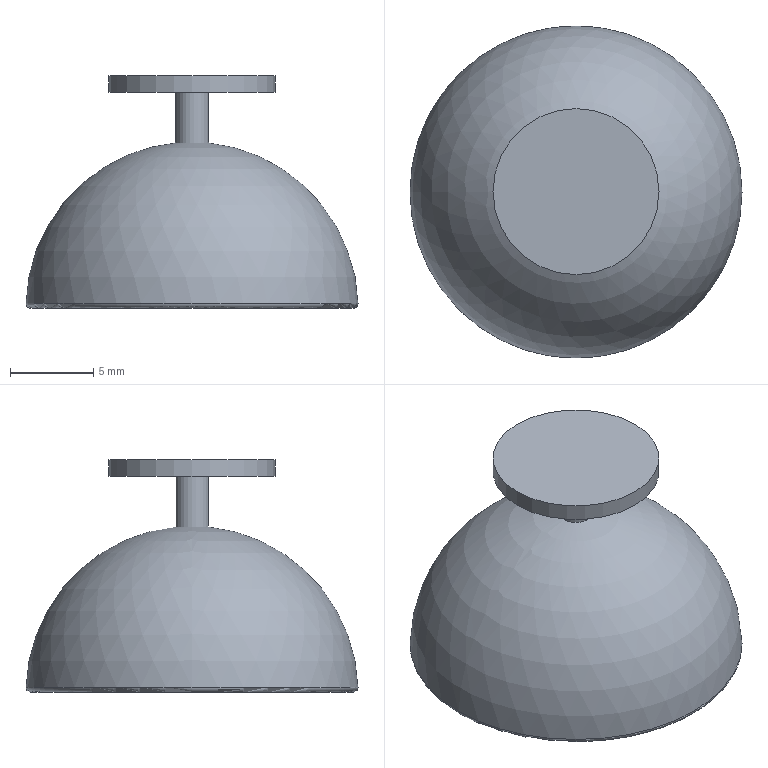Part | NX | features DATUM_CSYS 3, SKETCH 2, BLEND 1, REPLACE_FACE 1, SHELL 1, SPHERE 1, SWP104 1, TRIM BODY 1, UNITE 1 | 1 solid | 9 faces | box 19.991 x 19.991 x 14 mm | volume 1108 mm3 | plane 3 | sphere 2 | cylinder 2 | torus 2 | commonest cylinder face diameters 2 x1 10 x1
STEP:
#1=CARTESIAN_POINT('',(-9.995,0.,0.3093));
#2=VERTEX_POINT('',#1);
#3=CARTESIAN_POINT('',(0.,0.,0.3093));
#4=DIRECTION('',(0.,0.,-1.));
#5=DIRECTION('',(-1.,0.,0.));
#6=AXIS2_PLACEMENT_3D('',#3,#4,#5);
#7=CIRCLE('',#6,9.995);
#8=EDGE_CURVE('',#2,#2,#7,.F.);
#9=ORIENTED_EDGE('',*,*,#8,.T.);
#10=EDGE_LOOP('',(#9));
#11=FACE_BOUND('',#10,.T.);
#12=CARTESIAN_POINT('',(-1.,0.,9.95));
#13=VERTEX_POINT('',#12);
#14=CARTESIAN_POINT('',(0.,0.,9.95));
#15=DIRECTION('',(0.,0.,-1.));
#16=DIRECTION('',(-1.,0.,0.));
#17=AXIS2_PLACEMENT_3D('',#14,#15,#16);
#18=CIRCLE('',#17,1.);
#19=EDGE_CURVE('',#13,#13,#18,.T.);
#20=ORIENTED_EDGE('',*,*,#19,.T.);
#21=EDGE_LOOP('',(#20));
#22=FACE_BOUND('',#21,.T.);
#23=CARTESIAN_POINT('',(0.,0.,0.));
#24=DIRECTION('',(0.,0.,1.));
#25=DIRECTION('',(1.,0.,0.));
#26=AXIS2_PLACEMENT_3D('',#23,#24,#25);
#27=SPHERICAL_SURFACE('',#26,10.);
#28=ADVANCED_FACE('',(#11,#22),#27,.T.);
#29=CARTESIAN_POINT('',(-7.995,0.,0.2892));
#30=VERTEX_POINT('',#29);
#31=CARTESIAN_POINT('',(0.,0.,0.2892));
#32=DIRECTION('',(0.,0.,-1.));
#33=DIRECTION('',(-1.,0.,0.));
#34=AXIS2_PLACEMENT_3D('',#31,#32,#33);
#35=CIRCLE('',#34,7.995);
#36=EDGE_CURVE('',#30,#30,#35,.T.);
#37=ORIENTED_EDGE('',*,*,#36,.T.);
#38=EDGE_LOOP('',(#37));
#39=FACE_BOUND('',#38,.T.);
#40=CARTESIAN_POINT('',(0.,0.,0.));
#41=DIRECTION('',(0.,0.,1.));
#42=DIRECTION('',(1.,0.,0.));
#43=AXIS2_PLACEMENT_3D('',#40,#41,#42);
#44=SPHERICAL_SURFACE('',#43,8.);
#45=ADVANCED_FACE('',(#39),#44,.F.);
#46=CARTESIAN_POINT('',(8.295,0.,0.));
#47=VERTEX_POINT('',#46);
#48=CARTESIAN_POINT('',(0.,0.,0.));
#49=DIRECTION('',(0.,0.,1.));
#50=DIRECTION('',(1.,0.,0.));
#51=AXIS2_PLACEMENT_3D('',#48,#49,#50);
#52=CIRCLE('',#51,8.295);
#53=EDGE_CURVE('',#47,#47,#52,.T.);
#54=ORIENTED_EDGE('',*,*,#53,.T.);
#55=EDGE_LOOP('',(#54));
#56=FACE_BOUND('',#55,.T.);
#57=CARTESIAN_POINT('',(9.695,0.,0.));
#58=VERTEX_POINT('',#57);
#59=CARTESIAN_POINT('',(0.,0.,0.));
#60=DIRECTION('',(0.,0.,1.));
#61=DIRECTION('',(1.,0.,0.));
#62=AXIS2_PLACEMENT_3D('',#59,#60,#61);
#63=CIRCLE('',#62,9.695);
#64=EDGE_CURVE('',#58,#58,#63,.F.);
#65=ORIENTED_EDGE('',*,*,#64,.T.);
#66=EDGE_LOOP('',(#65));
#67=FACE_BOUND('',#66,.T.);
#68=CARTESIAN_POINT('',(0.,0.,0.));
#69=DIRECTION('',(0.,0.,1.));
#70=DIRECTION('',(1.,0.,0.));
#71=AXIS2_PLACEMENT_3D('',#68,#69,#70);
#72=PLANE('',#71);
#73=ADVANCED_FACE('',(#56,#67),#72,.F.);
#74=CARTESIAN_POINT('',(-5.,0.,14.));
#75=VERTEX_POINT('',#74);
#76=CARTESIAN_POINT('',(0.,0.,14.));
#77=DIRECTION('',(0.,0.,-1.));
#78=DIRECTION('',(-1.,0.,0.));
#79=AXIS2_PLACEMENT_3D('',#76,#77,#78);
#80=CIRCLE('',#79,5.);
#81=EDGE_CURVE('',#75,#75,#80,.T.);
#82=ORIENTED_EDGE('',*,*,#81,.F.);
#83=EDGE_LOOP('',(#82));
#84=FACE_BOUND('',#83,.T.);
#85=CARTESIAN_POINT('',(0.,0.,14.));
#86=DIRECTION('',(0.,0.,-1.));
#87=DIRECTION('',(-1.,0.,0.));
#88=AXIS2_PLACEMENT_3D('',#85,#86,#87);
#89=PLANE('',#88);
#90=ADVANCED_FACE('',(#84),#89,.F.);
#91=CARTESIAN_POINT('',(-5.,0.,13.));
#92=VERTEX_POINT('',#91);
#93=CARTESIAN_POINT('',(0.,0.,13.));
#94=DIRECTION('',(0.,0.,-1.));
#95=DIRECTION('',(-1.,0.,0.));
#96=AXIS2_PLACEMENT_3D('',#93,#94,#95);
#97=CIRCLE('',#96,5.);
#98=EDGE_CURVE('',#92,#92,#97,.T.);
#99=ORIENTED_EDGE('',*,*,#98,.F.);
#100=EDGE_LOOP('',(#99));
#101=FACE_BOUND('',#100,.T.);
#102=ORIENTED_EDGE('',*,*,#81,.T.);
#103=EDGE_LOOP('',(#102));
#104=FACE_BOUND('',#103,.T.);
#105=CARTESIAN_POINT('',(0.,0.,0.));
#106=DIRECTION('',(0.,0.,-1.));
#107=DIRECTION('',(-1.,0.,0.));
#108=AXIS2_PLACEMENT_3D('',#105,#106,#107);
#109=CYLINDRICAL_SURFACE('',#108,5.);
#110=ADVANCED_FACE('',(#101,#104),#109,.T.);
#111=CARTESIAN_POINT('',(-1.,0.,13.));
#112=VERTEX_POINT('',#111);
#113=CARTESIAN_POINT('',(0.,0.,13.));
#114=DIRECTION('',(0.,0.,-1.));
#115=DIRECTION('',(-1.,0.,0.));
#116=AXIS2_PLACEMENT_3D('',#113,#114,#115);
#117=CIRCLE('',#116,1.);
#118=EDGE_CURVE('',#112,#112,#117,.T.);
#119=ORIENTED_EDGE('',*,*,#118,.F.);
#120=EDGE_LOOP('',(#119));
#121=FACE_BOUND('',#120,.T.);
#122=ORIENTED_EDGE('',*,*,#98,.T.);
#123=EDGE_LOOP('',(#122));
#124=FACE_BOUND('',#123,.T.);
#125=CARTESIAN_POINT('',(5.,0.,13.));
#126=DIRECTION('',(0.,0.,1.));
#127=DIRECTION('',(1.,0.,0.));
#128=AXIS2_PLACEMENT_3D('',#125,#126,#127);
#129=PLANE('',#128);
#130=ADVANCED_FACE('',(#121,#124),#129,.F.);
#131=ORIENTED_EDGE('',*,*,#19,.F.);
#132=EDGE_LOOP('',(#131));
#133=FACE_BOUND('',#132,.T.);
#134=ORIENTED_EDGE('',*,*,#118,.T.);
#135=EDGE_LOOP('',(#134));
#136=FACE_BOUND('',#135,.T.);
#137=CARTESIAN_POINT('',(0.,0.,0.));
#138=DIRECTION('',(0.,0.,-1.));
#139=DIRECTION('',(-1.,0.,0.));
#140=AXIS2_PLACEMENT_3D('',#137,#138,#139);
#141=CYLINDRICAL_SURFACE('',#140,1.);
#142=ADVANCED_FACE('',(#133,#136),#141,.T.);
#143=ORIENTED_EDGE('',*,*,#53,.F.);
#144=EDGE_LOOP('',(#143));
#145=FACE_BOUND('',#144,.T.);
#146=ORIENTED_EDGE('',*,*,#36,.F.);
#147=EDGE_LOOP('',(#146));
#148=FACE_BOUND('',#147,.T.);
#149=CARTESIAN_POINT('',(0.,0.,0.3));
#150=DIRECTION('',(0.,0.,1.));
#151=DIRECTION('',(1.,0.,0.));
#152=AXIS2_PLACEMENT_3D('',#149,#150,#151);
#153=TOROIDAL_SURFACE('',#152,8.295,0.3);
#154=ADVANCED_FACE('',(#145,#148),#153,.T.);
#155=ORIENTED_EDGE('',*,*,#8,.F.);
#156=EDGE_LOOP('',(#155));
#157=FACE_BOUND('',#156,.T.);
#158=ORIENTED_EDGE('',*,*,#64,.F.);
#159=EDGE_LOOP('',(#158));
#160=FACE_BOUND('',#159,.T.);
#161=CARTESIAN_POINT('',(0.,0.,0.3));
#162=DIRECTION('',(0.,0.,1.));
#163=DIRECTION('',(1.,0.,0.));
#164=AXIS2_PLACEMENT_3D('',#161,#162,#163);
#165=TOROIDAL_SURFACE('',#164,9.695,0.3);
#166=ADVANCED_FACE('',(#157,#160),#165,.T.);
#167=CLOSED_SHELL('',(#28,#45,#73,#90,#110,#130,#142,#154,#166));
#168=MANIFOLD_SOLID_BREP('',#167);
#169=(LENGTH_UNIT()NAMED_UNIT(*)SI_UNIT(.MILLI.,.METRE.));
#170=UNCERTAINTY_MEASURE_WITH_UNIT(LENGTH_MEASURE(0.00001),#169,'','');
#171=(NAMED_UNIT(*)PLANE_ANGLE_UNIT()SI_UNIT($,.RADIAN.));
#172=(NAMED_UNIT(*)SI_UNIT($,.STERADIAN.)SOLID_ANGLE_UNIT());
#173=(GEOMETRIC_REPRESENTATION_CONTEXT(3)GLOBAL_UNCERTAINTY_ASSIGNED_CONTEXT((#170))GLOBAL_UNIT_ASSIGNED_CONTEXT((#169,#171,#172))REPRESENTATION_CONTEXT('',''));
#174=ADVANCED_BREP_SHAPE_REPRESENTATION('',(#168),#173);